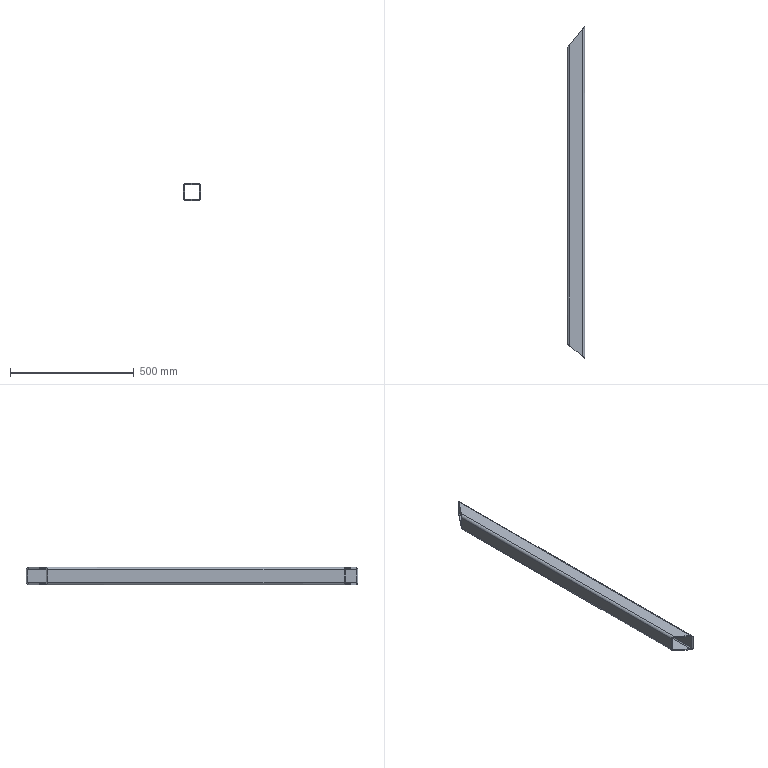Part | SolidWorks | features ICE 1, WeldMemberFeat 1, WeldmentFeature 1 | 1 solid | 18 faces | box 70 x 1340 x 70 mm | volume 1567074 mm3 | plane 10 | cylinder 8 | commonest cylinder face diameters 10 x4 20 x4
STEP:
#1=CARTESIAN_POINT('',(35.,0.,25.));
#2=VERTEX_POINT('',#1);
#3=CARTESIAN_POINT('',(35.,0.,-25.));
#4=VERTEX_POINT('',#3);
#5=CARTESIAN_POINT('',(35.,0.,-25.));
#6=DIRECTION('',(0.,0.,-1.));
#7=VECTOR('',#6,1000.);
#8=LINE('',#5,#7);
#9=EDGE_CURVE('',#2,#4,#8,.T.);
#10=ORIENTED_EDGE('',*,*,#9,.T.);
#11=CARTESIAN_POINT('',(35.,1340.,-25.));
#12=VERTEX_POINT('',#11);
#13=CARTESIAN_POINT('',(35.,1340.,-25.));
#14=DIRECTION('',(0.,-1.,0.));
#15=VECTOR('',#14,1000.);
#16=LINE('',#13,#15);
#17=EDGE_CURVE('',#12,#4,#16,.T.);
#18=ORIENTED_EDGE('',*,*,#17,.F.);
#19=CARTESIAN_POINT('',(35.,1340.,25.));
#20=VERTEX_POINT('',#19);
#21=CARTESIAN_POINT('',(35.,1340.,-25.));
#22=DIRECTION('',(0.,0.,-1.));
#23=VECTOR('',#22,1000.);
#24=LINE('',#21,#23);
#25=EDGE_CURVE('',#20,#12,#24,.T.);
#26=ORIENTED_EDGE('',*,*,#25,.F.);
#27=CARTESIAN_POINT('',(35.,1340.,25.));
#28=DIRECTION('',(0.,-1.,0.));
#29=VECTOR('',#28,1000.);
#30=LINE('',#27,#29);
#31=EDGE_CURVE('',#20,#2,#30,.T.);
#32=ORIENTED_EDGE('',*,*,#31,.T.);
#33=EDGE_LOOP('',(#10,#18,#26,#32));
#34=FACE_OUTER_BOUND('',#33,.T.);
#35=CARTESIAN_POINT('',(35.,1340.,-25.));
#36=DIRECTION('',(-1.,0.,0.));
#37=DIRECTION('',(0.,0.,1.));
#38=AXIS2_PLACEMENT_3D('',#35,#36,#37);
#39=PLANE('',#38);
#40=ADVANCED_FACE('',(#34),#39,.F.);
#41=CARTESIAN_POINT('',(-35.,1252.5,25.));
#42=VERTEX_POINT('',#41);
#43=CARTESIAN_POINT('',(-35.,56.,25.));
#44=VERTEX_POINT('',#43);
#45=CARTESIAN_POINT('',(-35.,1340.,25.));
#46=DIRECTION('',(0.,-1.,0.));
#47=VECTOR('',#46,1000.);
#48=LINE('',#45,#47);
#49=EDGE_CURVE('',#42,#44,#48,.T.);
#50=ORIENTED_EDGE('',*,*,#49,.F.);
#51=CARTESIAN_POINT('',(-35.,1252.5,-25.));
#52=VERTEX_POINT('',#51);
#53=CARTESIAN_POINT('',(-35.,1252.5,-35.));
#54=DIRECTION('',(0.,0.,1.));
#55=VECTOR('',#54,1000.);
#56=LINE('',#53,#55);
#57=EDGE_CURVE('',#52,#42,#56,.T.);
#58=ORIENTED_EDGE('',*,*,#57,.F.);
#59=CARTESIAN_POINT('',(-35.,56.,-25.));
#60=VERTEX_POINT('',#59);
#61=CARTESIAN_POINT('',(-35.,1340.,-25.));
#62=DIRECTION('',(0.,-1.,0.));
#63=VECTOR('',#62,1000.);
#64=LINE('',#61,#63);
#65=EDGE_CURVE('',#52,#60,#64,.T.);
#66=ORIENTED_EDGE('',*,*,#65,.T.);
#67=CARTESIAN_POINT('',(-35.,56.,-35.));
#68=DIRECTION('',(0.,0.,1.));
#69=VECTOR('',#68,1000.);
#70=LINE('',#67,#69);
#71=EDGE_CURVE('',#60,#44,#70,.T.);
#72=ORIENTED_EDGE('',*,*,#71,.T.);
#73=EDGE_LOOP('',(#50,#58,#66,#72));
#74=FACE_OUTER_BOUND('',#73,.T.);
#75=CARTESIAN_POINT('',(-35.,1340.,25.));
#76=DIRECTION('',(1.,0.,0.));
#77=DIRECTION('',(0.,0.,-1.));
#78=AXIS2_PLACEMENT_3D('',#75,#76,#77);
#79=PLANE('',#78);
#80=ADVANCED_FACE('',(#74),#79,.F.);
#81=ORIENTED_EDGE('',*,*,#65,.F.);
#82=CARTESIAN_POINT('',(-25.,1265.,-35.));
#83=VERTEX_POINT('',#82);
#84=CARTESIAN_POINT('',(-35.,1252.5,-25.));
#85=CARTESIAN_POINT('',(-35.,1252.5,-30.858));
#86=CARTESIAN_POINT('',(-30.858,1257.678,-35.));
#87=CARTESIAN_POINT('',(-25.,1265.,-35.));
#88=(BOUNDED_CURVE()B_SPLINE_CURVE(3,(#84,#85,#86,#87),.UNSPECIFIED.,.F.,.T.)B_SPLINE_CURVE_WITH_KNOTS((4,4),(0.,1.571),.UNSPECIFIED.)CURVE()GEOMETRIC_REPRESENTATION_ITEM()RATIONAL_B_SPLINE_CURVE((1.,0.8047,0.8047,1.))REPRESENTATION_ITEM(''));
#89=EDGE_CURVE('',#52,#83,#88,.T.);
#90=ORIENTED_EDGE('',*,*,#89,.T.);
#91=CARTESIAN_POINT('',(-25.,48.,-35.));
#92=VERTEX_POINT('',#91);
#93=CARTESIAN_POINT('',(-25.,1340.,-35.));
#94=DIRECTION('',(0.,-1.,0.));
#95=VECTOR('',#94,1000.);
#96=LINE('',#93,#95);
#97=EDGE_CURVE('',#83,#92,#96,.T.);
#98=ORIENTED_EDGE('',*,*,#97,.T.);
#99=CARTESIAN_POINT('',(-25.,48.,-35.));
#100=CARTESIAN_POINT('',(-30.858,52.686,-35.));
#101=CARTESIAN_POINT('',(-35.,56.,-30.858));
#102=CARTESIAN_POINT('',(-35.,56.,-25.));
#103=(BOUNDED_CURVE()B_SPLINE_CURVE(3,(#99,#100,#101,#102),.UNSPECIFIED.,.F.,.T.)B_SPLINE_CURVE_WITH_KNOTS((4,4),(1.571,3.142),.UNSPECIFIED.)CURVE()GEOMETRIC_REPRESENTATION_ITEM()RATIONAL_B_SPLINE_CURVE((1.,0.8047,0.8047,1.))REPRESENTATION_ITEM(''));
#104=EDGE_CURVE('',#92,#60,#103,.T.);
#105=ORIENTED_EDGE('',*,*,#104,.T.);
#106=EDGE_LOOP('',(#81,#90,#98,#105));
#107=FACE_OUTER_BOUND('',#106,.T.);
#108=CARTESIAN_POINT('',(-25.,1340.,-25.));
#109=DIRECTION('',(0.,-1.,0.));
#110=DIRECTION('',(0.,0.,-1.));
#111=AXIS2_PLACEMENT_3D('',#108,#109,#110);
#112=CYLINDRICAL_SURFACE('',#111,10.);
#113=ADVANCED_FACE('',(#107),#112,.T.);
#114=ORIENTED_EDGE('',*,*,#97,.F.);
#115=CARTESIAN_POINT('',(25.,1327.5,-35.));
#116=VERTEX_POINT('',#115);
#117=CARTESIAN_POINT('',(35.,1340.,-35.));
#118=DIRECTION('',(0.6247,0.7809,0.));
#119=VECTOR('',#118,1000.);
#120=LINE('',#117,#119);
#121=EDGE_CURVE('',#83,#116,#120,.T.);
#122=ORIENTED_EDGE('',*,*,#121,.T.);
#123=CARTESIAN_POINT('',(25.,8.,-35.));
#124=VERTEX_POINT('',#123);
#125=CARTESIAN_POINT('',(25.,1340.,-35.));
#126=DIRECTION('',(0.,-1.,0.));
#127=VECTOR('',#126,1000.);
#128=LINE('',#125,#127);
#129=EDGE_CURVE('',#116,#124,#128,.T.);
#130=ORIENTED_EDGE('',*,*,#129,.T.);
#131=CARTESIAN_POINT('',(-35.,56.,-35.));
#132=DIRECTION('',(-0.7809,0.6247,0.));
#133=VECTOR('',#132,1000.);
#134=LINE('',#131,#133);
#135=EDGE_CURVE('',#124,#92,#134,.T.);
#136=ORIENTED_EDGE('',*,*,#135,.T.);
#137=EDGE_LOOP('',(#114,#122,#130,#136));
#138=FACE_OUTER_BOUND('',#137,.T.);
#139=CARTESIAN_POINT('',(25.,1340.,-35.));
#140=DIRECTION('',(0.,0.,1.));
#141=DIRECTION('',(1.,0.,0.));
#142=AXIS2_PLACEMENT_3D('',#139,#140,#141);
#143=PLANE('',#142);
#144=ADVANCED_FACE('',(#138),#143,.F.);
#145=ORIENTED_EDGE('',*,*,#129,.F.);
#146=CARTESIAN_POINT('',(25.,1327.5,-35.));
#147=CARTESIAN_POINT('',(30.858,1334.822,-35.));
#148=CARTESIAN_POINT('',(35.,1340.,-30.858));
#149=CARTESIAN_POINT('',(35.,1340.,-25.));
#150=(BOUNDED_CURVE()B_SPLINE_CURVE(3,(#146,#147,#148,#149),.UNSPECIFIED.,.F.,.F.)B_SPLINE_CURVE_WITH_KNOTS((4,4),(1.571,3.142),.UNSPECIFIED.)CURVE()GEOMETRIC_REPRESENTATION_ITEM()RATIONAL_B_SPLINE_CURVE((1.,0.8047,0.8047,1.))REPRESENTATION_ITEM(''));
#151=EDGE_CURVE('',#116,#12,#150,.T.);
#152=ORIENTED_EDGE('',*,*,#151,.T.);
#153=ORIENTED_EDGE('',*,*,#17,.T.);
#154=CARTESIAN_POINT('',(35.,0.,-25.));
#155=CARTESIAN_POINT('',(35.,0.,-30.858));
#156=CARTESIAN_POINT('',(30.858,3.314,-35.));
#157=CARTESIAN_POINT('',(25.,8.,-35.));
#158=(BOUNDED_CURVE()B_SPLINE_CURVE(3,(#154,#155,#156,#157),.UNSPECIFIED.,.F.,.F.)B_SPLINE_CURVE_WITH_KNOTS((4,4),(0.,1.571),.UNSPECIFIED.)CURVE()GEOMETRIC_REPRESENTATION_ITEM()RATIONAL_B_SPLINE_CURVE((1.,0.8047,0.8047,1.))REPRESENTATION_ITEM(''));
#159=EDGE_CURVE('',#4,#124,#158,.T.);
#160=ORIENTED_EDGE('',*,*,#159,.T.);
#161=EDGE_LOOP('',(#145,#152,#153,#160));
#162=FACE_OUTER_BOUND('',#161,.T.);
#163=CARTESIAN_POINT('',(25.,1340.,-25.));
#164=DIRECTION('',(0.,-1.,0.));
#165=DIRECTION('',(0.,0.,-1.));
#166=AXIS2_PLACEMENT_3D('',#163,#164,#165);
#167=CYLINDRICAL_SURFACE('',#166,10.);
#168=ADVANCED_FACE('',(#162),#167,.T.);
#169=ORIENTED_EDGE('',*,*,#31,.F.);
#170=CARTESIAN_POINT('',(25.,1327.5,35.));
#171=VERTEX_POINT('',#170);
#172=CARTESIAN_POINT('',(35.,1340.,25.));
#173=CARTESIAN_POINT('',(35.,1340.,30.858));
#174=CARTESIAN_POINT('',(30.858,1334.822,35.));
#175=CARTESIAN_POINT('',(25.,1327.5,35.));
#176=(BOUNDED_CURVE()B_SPLINE_CURVE(3,(#172,#173,#174,#175),.UNSPECIFIED.,.F.,.T.)B_SPLINE_CURVE_WITH_KNOTS((4,4),(3.142,4.712),.UNSPECIFIED.)CURVE()GEOMETRIC_REPRESENTATION_ITEM()RATIONAL_B_SPLINE_CURVE((1.,0.8047,0.8047,1.))REPRESENTATION_ITEM(''));
#177=EDGE_CURVE('',#20,#171,#176,.T.);
#178=ORIENTED_EDGE('',*,*,#177,.T.);
#179=CARTESIAN_POINT('',(25.,8.,35.));
#180=VERTEX_POINT('',#179);
#181=CARTESIAN_POINT('',(25.,1340.,35.));
#182=DIRECTION('',(0.,-1.,0.));
#183=VECTOR('',#182,1000.);
#184=LINE('',#181,#183);
#185=EDGE_CURVE('',#171,#180,#184,.T.);
#186=ORIENTED_EDGE('',*,*,#185,.T.);
#187=CARTESIAN_POINT('',(25.,8.,35.));
#188=CARTESIAN_POINT('',(30.858,3.314,35.));
#189=CARTESIAN_POINT('',(35.,0.,30.858));
#190=CARTESIAN_POINT('',(35.,0.,25.));
#191=(BOUNDED_CURVE()B_SPLINE_CURVE(3,(#187,#188,#189,#190),.UNSPECIFIED.,.F.,.F.)B_SPLINE_CURVE_WITH_KNOTS((4,4),(4.712,6.283),.UNSPECIFIED.)CURVE()GEOMETRIC_REPRESENTATION_ITEM()RATIONAL_B_SPLINE_CURVE((1.,0.8047,0.8047,1.))REPRESENTATION_ITEM(''));
#192=EDGE_CURVE('',#180,#2,#191,.T.);
#193=ORIENTED_EDGE('',*,*,#192,.T.);
#194=EDGE_LOOP('',(#169,#178,#186,#193));
#195=FACE_OUTER_BOUND('',#194,.T.);
#196=CARTESIAN_POINT('',(25.,1340.,25.));
#197=DIRECTION('',(0.,-1.,0.));
#198=DIRECTION('',(0.,0.,-1.));
#199=AXIS2_PLACEMENT_3D('',#196,#197,#198);
#200=CYLINDRICAL_SURFACE('',#199,10.);
#201=ADVANCED_FACE('',(#195),#200,.T.);
#202=ORIENTED_EDGE('',*,*,#185,.F.);
#203=CARTESIAN_POINT('',(-25.,1265.,35.));
#204=VERTEX_POINT('',#203);
#205=CARTESIAN_POINT('',(11.585,1310.732,35.));
#206=DIRECTION('',(-0.6247,-0.7809,0.));
#207=VECTOR('',#206,1000.);
#208=LINE('',#205,#207);
#209=EDGE_CURVE('',#171,#204,#208,.T.);
#210=ORIENTED_EDGE('',*,*,#209,.T.);
#211=CARTESIAN_POINT('',(-25.,48.,35.));
#212=VERTEX_POINT('',#211);
#213=CARTESIAN_POINT('',(-25.,1340.,35.));
#214=DIRECTION('',(0.,-1.,0.));
#215=VECTOR('',#214,1000.);
#216=LINE('',#213,#215);
#217=EDGE_CURVE('',#204,#212,#216,.T.);
#218=ORIENTED_EDGE('',*,*,#217,.T.);
#219=CARTESIAN_POINT('',(-655.244,552.195,35.));
#220=DIRECTION('',(0.7809,-0.6247,0.));
#221=VECTOR('',#220,1000.);
#222=LINE('',#219,#221);
#223=EDGE_CURVE('',#212,#180,#222,.T.);
#224=ORIENTED_EDGE('',*,*,#223,.T.);
#225=EDGE_LOOP('',(#202,#210,#218,#224));
#226=FACE_OUTER_BOUND('',#225,.T.);
#227=CARTESIAN_POINT('',(-25.,1340.,35.));
#228=DIRECTION('',(0.,0.,-1.));
#229=DIRECTION('',(-1.,0.,0.));
#230=AXIS2_PLACEMENT_3D('',#227,#228,#229);
#231=PLANE('',#230);
#232=ADVANCED_FACE('',(#226),#231,.F.);
#233=ORIENTED_EDGE('',*,*,#217,.F.);
#234=CARTESIAN_POINT('',(-25.,1265.,35.));
#235=CARTESIAN_POINT('',(-30.858,1257.678,35.));
#236=CARTESIAN_POINT('',(-35.,1252.5,30.858));
#237=CARTESIAN_POINT('',(-35.,1252.5,25.));
#238=(BOUNDED_CURVE()B_SPLINE_CURVE(3,(#234,#235,#236,#237),.UNSPECIFIED.,.F.,.F.)B_SPLINE_CURVE_WITH_KNOTS((4,4),(4.712,6.283),.UNSPECIFIED.)CURVE()GEOMETRIC_REPRESENTATION_ITEM()RATIONAL_B_SPLINE_CURVE((1.,0.8047,0.8047,1.))REPRESENTATION_ITEM(''));
#239=EDGE_CURVE('',#204,#42,#238,.T.);
#240=ORIENTED_EDGE('',*,*,#239,.T.);
#241=ORIENTED_EDGE('',*,*,#49,.T.);
#242=CARTESIAN_POINT('',(-35.,56.,25.));
#243=CARTESIAN_POINT('',(-35.,56.,30.858));
#244=CARTESIAN_POINT('',(-30.858,52.686,35.));
#245=CARTESIAN_POINT('',(-25.,48.,35.));
#246=(BOUNDED_CURVE()B_SPLINE_CURVE(3,(#242,#243,#244,#245),.UNSPECIFIED.,.F.,.F.)B_SPLINE_CURVE_WITH_KNOTS((4,4),(3.142,4.712),.UNSPECIFIED.)CURVE()GEOMETRIC_REPRESENTATION_ITEM()RATIONAL_B_SPLINE_CURVE((1.,0.8047,0.8047,1.))REPRESENTATION_ITEM(''));
#247=EDGE_CURVE('',#44,#212,#246,.T.);
#248=ORIENTED_EDGE('',*,*,#247,.T.);
#249=EDGE_LOOP('',(#233,#240,#241,#248));
#250=FACE_OUTER_BOUND('',#249,.T.);
#251=CARTESIAN_POINT('',(-25.,1340.,25.));
#252=DIRECTION('',(0.,-1.,0.));
#253=DIRECTION('',(0.,0.,-1.));
#254=AXIS2_PLACEMENT_3D('',#251,#252,#253);
#255=CYLINDRICAL_SURFACE('',#254,10.);
#256=ADVANCED_FACE('',(#250),#255,.T.);
#257=CARTESIAN_POINT('',(25.,8.,30.));
#258=VERTEX_POINT('',#257);
#259=CARTESIAN_POINT('',(30.,4.,25.));
#260=VERTEX_POINT('',#259);
#261=CARTESIAN_POINT('',(25.,8.,30.));
#262=CARTESIAN_POINT('',(27.929,5.657,30.));
#263=CARTESIAN_POINT('',(30.,4.,27.929));
#264=CARTESIAN_POINT('',(30.,4.,25.));
#265=(BOUNDED_CURVE()B_SPLINE_CURVE(3,(#261,#262,#263,#264),.UNSPECIFIED.,.F.,.F.)B_SPLINE_CURVE_WITH_KNOTS((4,4),(4.712,6.283),.UNSPECIFIED.)CURVE()GEOMETRIC_REPRESENTATION_ITEM()RATIONAL_B_SPLINE_CURVE((1.,0.8047,0.8047,1.))REPRESENTATION_ITEM(''));
#266=EDGE_CURVE('',#258,#260,#265,.T.);
#267=ORIENTED_EDGE('',*,*,#266,.T.);
#268=CARTESIAN_POINT('',(30.,4.,-25.));
#269=VERTEX_POINT('',#268);
#270=CARTESIAN_POINT('',(30.,4.,-25.));
#271=DIRECTION('',(0.,0.,-1.));
#272=VECTOR('',#271,1000.);
#273=LINE('',#270,#272);
#274=EDGE_CURVE('',#260,#269,#273,.T.);
#275=ORIENTED_EDGE('',*,*,#274,.T.);
#276=CARTESIAN_POINT('',(25.,8.,-30.));
#277=VERTEX_POINT('',#276);
#278=CARTESIAN_POINT('',(30.,4.,-25.));
#279=CARTESIAN_POINT('',(30.,4.,-27.929));
#280=CARTESIAN_POINT('',(27.929,5.657,-30.));
#281=CARTESIAN_POINT('',(25.,8.,-30.));
#282=(BOUNDED_CURVE()B_SPLINE_CURVE(3,(#278,#279,#280,#281),.UNSPECIFIED.,.F.,.F.)B_SPLINE_CURVE_WITH_KNOTS((4,4),(0.,1.571),.UNSPECIFIED.)CURVE()GEOMETRIC_REPRESENTATION_ITEM()RATIONAL_B_SPLINE_CURVE((1.,0.8047,0.8047,1.))REPRESENTATION_ITEM(''));
#283=EDGE_CURVE('',#269,#277,#282,.T.);
#284=ORIENTED_EDGE('',*,*,#283,.T.);
#285=CARTESIAN_POINT('',(-25.,48.,-30.));
#286=VERTEX_POINT('',#285);
#287=CARTESIAN_POINT('',(-624.756,527.805,-30.));
#288=DIRECTION('',(-0.7809,0.6247,0.));
#289=VECTOR('',#288,1000.);
#290=LINE('',#287,#289);
#291=EDGE_CURVE('',#277,#286,#290,.T.);
#292=ORIENTED_EDGE('',*,*,#291,.T.);
#293=CARTESIAN_POINT('',(-30.,52.,-25.));
#294=VERTEX_POINT('',#293);
#295=CARTESIAN_POINT('',(-25.,48.,-30.));
#296=CARTESIAN_POINT('',(-27.929,50.343,-30.));
#297=CARTESIAN_POINT('',(-30.,52.,-27.929));
#298=CARTESIAN_POINT('',(-30.,52.,-25.));
#299=(BOUNDED_CURVE()B_SPLINE_CURVE(3,(#295,#296,#297,#298),.UNSPECIFIED.,.F.,.F.)B_SPLINE_CURVE_WITH_KNOTS((4,4),(1.571,3.142),.UNSPECIFIED.)CURVE()GEOMETRIC_REPRESENTATION_ITEM()RATIONAL_B_SPLINE_CURVE((1.,0.8047,0.8047,1.))REPRESENTATION_ITEM(''));
#300=EDGE_CURVE('',#286,#294,#299,.T.);
#301=ORIENTED_EDGE('',*,*,#300,.T.);
#302=CARTESIAN_POINT('',(-30.,52.,25.));
#303=VERTEX_POINT('',#302);
#304=CARTESIAN_POINT('',(-30.,52.,25.));
#305=DIRECTION('',(0.,0.,1.));
#306=VECTOR('',#305,1000.);
#307=LINE('',#304,#306);
#308=EDGE_CURVE('',#294,#303,#307,.T.);
#309=ORIENTED_EDGE('',*,*,#308,.T.);
#310=CARTESIAN_POINT('',(-25.,48.,30.));
#311=VERTEX_POINT('',#310);
#312=CARTESIAN_POINT('',(-30.,52.,25.));
#313=CARTESIAN_POINT('',(-30.,52.,27.929));
#314=CARTESIAN_POINT('',(-27.929,50.343,30.));
#315=CARTESIAN_POINT('',(-25.,48.,30.));
#316=(BOUNDED_CURVE()B_SPLINE_CURVE(3,(#312,#313,#314,#315),.UNSPECIFIED.,.F.,.T.)B_SPLINE_CURVE_WITH_KNOTS((4,4),(3.142,4.712),.UNSPECIFIED.)CURVE()GEOMETRIC_REPRESENTATION_ITEM()RATIONAL_B_SPLINE_CURVE((1.,0.8047,0.8047,1.))REPRESENTATION_ITEM(''));
#317=EDGE_CURVE('',#303,#311,#316,.T.);
#318=ORIENTED_EDGE('',*,*,#317,.T.);
#319=CARTESIAN_POINT('',(-655.244,552.195,30.));
#320=DIRECTION('',(0.7809,-0.6247,0.));
#321=VECTOR('',#320,1000.);
#322=LINE('',#319,#321);
#323=EDGE_CURVE('',#311,#258,#322,.T.);
#324=ORIENTED_EDGE('',*,*,#323,.T.);
#325=EDGE_LOOP('',(#267,#275,#284,#292,#301,#309,#318,#324));
#326=FACE_BOUND('',#325,.T.);
#327=ORIENTED_EDGE('',*,*,#71,.F.);
#328=ORIENTED_EDGE('',*,*,#104,.F.);
#329=ORIENTED_EDGE('',*,*,#135,.F.);
#330=ORIENTED_EDGE('',*,*,#159,.F.);
#331=ORIENTED_EDGE('',*,*,#9,.F.);
#332=ORIENTED_EDGE('',*,*,#192,.F.);
#333=ORIENTED_EDGE('',*,*,#223,.F.);
#334=ORIENTED_EDGE('',*,*,#247,.F.);
#335=EDGE_LOOP('',(#327,#328,#329,#330,#331,#332,#333,#334));
#336=FACE_OUTER_BOUND('',#335,.T.);
#337=CARTESIAN_POINT('',(-35.,56.,-35.));
#338=DIRECTION('',(0.6247,0.7809,0.));
#339=DIRECTION('',(-0.7809,0.6247,0.));
#340=AXIS2_PLACEMENT_3D('',#337,#338,#339);
#341=PLANE('',#340);
#342=ADVANCED_FACE('',(#326,#336),#341,.F.);
#343=CARTESIAN_POINT('',(30.,1333.75,25.));
#344=VERTEX_POINT('',#343);
#345=CARTESIAN_POINT('',(25.,1327.5,30.));
#346=VERTEX_POINT('',#345);
#347=CARTESIAN_POINT('',(30.,1333.75,25.));
#348=CARTESIAN_POINT('',(30.,1333.75,27.929));
#349=CARTESIAN_POINT('',(27.929,1331.161,30.));
#350=CARTESIAN_POINT('',(25.,1327.5,30.));
#351=(BOUNDED_CURVE()B_SPLINE_CURVE(3,(#347,#348,#349,#350),.UNSPECIFIED.,.F.,.T.)B_SPLINE_CURVE_WITH_KNOTS((4,4),(3.142,4.712),.UNSPECIFIED.)CURVE()GEOMETRIC_REPRESENTATION_ITEM()RATIONAL_B_SPLINE_CURVE((1.,0.8047,0.8047,1.))REPRESENTATION_ITEM(''));
#352=EDGE_CURVE('',#344,#346,#351,.T.);
#353=ORIENTED_EDGE('',*,*,#352,.T.);
#354=CARTESIAN_POINT('',(-25.,1265.,30.));
#355=VERTEX_POINT('',#354);
#356=CARTESIAN_POINT('',(11.585,1310.732,30.));
#357=DIRECTION('',(-0.6247,-0.7809,0.));
#358=VECTOR('',#357,1000.);
#359=LINE('',#356,#358);
#360=EDGE_CURVE('',#346,#355,#359,.T.);
#361=ORIENTED_EDGE('',*,*,#360,.T.);
#362=CARTESIAN_POINT('',(-30.,1258.75,25.));
#363=VERTEX_POINT('',#362);
#364=CARTESIAN_POINT('',(-25.,1265.,30.));
#365=CARTESIAN_POINT('',(-27.929,1261.339,30.));
#366=CARTESIAN_POINT('',(-30.,1258.75,27.929));
#367=CARTESIAN_POINT('',(-30.,1258.75,25.));
#368=(BOUNDED_CURVE()B_SPLINE_CURVE(3,(#364,#365,#366,#367),.UNSPECIFIED.,.F.,.F.)B_SPLINE_CURVE_WITH_KNOTS((4,4),(4.712,6.283),.UNSPECIFIED.)CURVE()GEOMETRIC_REPRESENTATION_ITEM()RATIONAL_B_SPLINE_CURVE((1.,0.8047,0.8047,1.))REPRESENTATION_ITEM(''));
#369=EDGE_CURVE('',#355,#363,#368,.T.);
#370=ORIENTED_EDGE('',*,*,#369,.T.);
#371=CARTESIAN_POINT('',(-30.,1258.75,-25.));
#372=VERTEX_POINT('',#371);
#373=CARTESIAN_POINT('',(-30.,1258.75,25.));
#374=DIRECTION('',(0.,0.,-1.));
#375=VECTOR('',#374,1000.);
#376=LINE('',#373,#375);
#377=EDGE_CURVE('',#363,#372,#376,.T.);
#378=ORIENTED_EDGE('',*,*,#377,.T.);
#379=CARTESIAN_POINT('',(-25.,1265.,-30.));
#380=VERTEX_POINT('',#379);
#381=CARTESIAN_POINT('',(-30.,1258.75,-25.));
#382=CARTESIAN_POINT('',(-30.,1258.75,-27.929));
#383=CARTESIAN_POINT('',(-27.929,1261.339,-30.));
#384=CARTESIAN_POINT('',(-25.,1265.,-30.));
#385=(BOUNDED_CURVE()B_SPLINE_CURVE(3,(#381,#382,#383,#384),.UNSPECIFIED.,.F.,.F.)B_SPLINE_CURVE_WITH_KNOTS((4,4),(0.,1.571),.UNSPECIFIED.)CURVE()GEOMETRIC_REPRESENTATION_ITEM()RATIONAL_B_SPLINE_CURVE((1.,0.8047,0.8047,1.))REPRESENTATION_ITEM(''));
#386=EDGE_CURVE('',#372,#380,#385,.T.);
#387=ORIENTED_EDGE('',*,*,#386,.T.);
#388=CARTESIAN_POINT('',(25.,1327.5,-30.));
#389=VERTEX_POINT('',#388);
#390=CARTESIAN_POINT('',(31.098,1335.122,-30.));
#391=DIRECTION('',(0.6247,0.7809,0.));
#392=VECTOR('',#391,1000.);
#393=LINE('',#390,#392);
#394=EDGE_CURVE('',#380,#389,#393,.T.);
#395=ORIENTED_EDGE('',*,*,#394,.T.);
#396=CARTESIAN_POINT('',(30.,1333.75,-25.));
#397=VERTEX_POINT('',#396);
#398=CARTESIAN_POINT('',(25.,1327.5,-30.));
#399=CARTESIAN_POINT('',(27.929,1331.161,-30.));
#400=CARTESIAN_POINT('',(30.,1333.75,-27.929));
#401=CARTESIAN_POINT('',(30.,1333.75,-25.));
#402=(BOUNDED_CURVE()B_SPLINE_CURVE(3,(#398,#399,#400,#401),.UNSPECIFIED.,.F.,.F.)B_SPLINE_CURVE_WITH_KNOTS((4,4),(1.571,3.142),.UNSPECIFIED.)CURVE()GEOMETRIC_REPRESENTATION_ITEM()RATIONAL_B_SPLINE_CURVE((1.,0.8047,0.8047,1.))REPRESENTATION_ITEM(''));
#403=EDGE_CURVE('',#389,#397,#402,.T.);
#404=ORIENTED_EDGE('',*,*,#403,.T.);
#405=CARTESIAN_POINT('',(30.,1333.75,-25.));
#406=DIRECTION('',(0.,0.,1.));
#407=VECTOR('',#406,1000.);
#408=LINE('',#405,#407);
#409=EDGE_CURVE('',#397,#344,#408,.T.);
#410=ORIENTED_EDGE('',*,*,#409,.T.);
#411=EDGE_LOOP('',(#353,#361,#370,#378,#387,#395,#404,#410));
#412=FACE_BOUND('',#411,.T.);
#413=ORIENTED_EDGE('',*,*,#209,.F.);
#414=ORIENTED_EDGE('',*,*,#177,.F.);
#415=ORIENTED_EDGE('',*,*,#25,.T.);
#416=ORIENTED_EDGE('',*,*,#151,.F.);
#417=ORIENTED_EDGE('',*,*,#121,.F.);
#418=ORIENTED_EDGE('',*,*,#89,.F.);
#419=ORIENTED_EDGE('',*,*,#57,.T.);
#420=ORIENTED_EDGE('',*,*,#239,.F.);
#421=EDGE_LOOP('',(#413,#414,#415,#416,#417,#418,#419,#420));
#422=FACE_OUTER_BOUND('',#421,.T.);
#423=CARTESIAN_POINT('',(35.,1340.,-35.));
#424=DIRECTION('',(0.7809,-0.6247,0.));
#425=DIRECTION('',(0.6247,0.7809,0.));
#426=AXIS2_PLACEMENT_3D('',#423,#424,#425);
#427=PLANE('',#426);
#428=ADVANCED_FACE('',(#412,#422),#427,.F.);
#429=ORIENTED_EDGE('',*,*,#352,.F.);
#430=CARTESIAN_POINT('',(30.,1340.,25.));
#431=DIRECTION('',(0.,-1.,0.));
#432=VECTOR('',#431,1000.);
#433=LINE('',#430,#432);
#434=EDGE_CURVE('',#344,#260,#433,.T.);
#435=ORIENTED_EDGE('',*,*,#434,.T.);
#436=ORIENTED_EDGE('',*,*,#266,.F.);
#437=CARTESIAN_POINT('',(25.,1340.,30.));
#438=DIRECTION('',(0.,-1.,0.));
#439=VECTOR('',#438,1000.);
#440=LINE('',#437,#439);
#441=EDGE_CURVE('',#346,#258,#440,.T.);
#442=ORIENTED_EDGE('',*,*,#441,.F.);
#443=EDGE_LOOP('',(#429,#435,#436,#442));
#444=FACE_OUTER_BOUND('',#443,.T.);
#445=CARTESIAN_POINT('',(25.,1340.,25.));
#446=DIRECTION('',(0.,-1.,0.));
#447=DIRECTION('',(0.,0.,-1.));
#448=AXIS2_PLACEMENT_3D('',#445,#446,#447);
#449=CYLINDRICAL_SURFACE('',#448,5.);
#450=ADVANCED_FACE('',(#444),#449,.F.);
#451=ORIENTED_EDGE('',*,*,#360,.F.);
#452=ORIENTED_EDGE('',*,*,#441,.T.);
#453=ORIENTED_EDGE('',*,*,#323,.F.);
#454=CARTESIAN_POINT('',(-25.,1340.,30.));
#455=DIRECTION('',(0.,-1.,0.));
#456=VECTOR('',#455,1000.);
#457=LINE('',#454,#456);
#458=EDGE_CURVE('',#355,#311,#457,.T.);
#459=ORIENTED_EDGE('',*,*,#458,.F.);
#460=EDGE_LOOP('',(#451,#452,#453,#459));
#461=FACE_OUTER_BOUND('',#460,.T.);
#462=CARTESIAN_POINT('',(-25.,1340.,30.));
#463=DIRECTION('',(0.,0.,-1.));
#464=DIRECTION('',(-1.,0.,0.));
#465=AXIS2_PLACEMENT_3D('',#462,#463,#464);
#466=PLANE('',#465);
#467=ADVANCED_FACE('',(#461),#466,.T.);
#468=ORIENTED_EDGE('',*,*,#369,.F.);
#469=ORIENTED_EDGE('',*,*,#458,.T.);
#470=ORIENTED_EDGE('',*,*,#317,.F.);
#471=CARTESIAN_POINT('',(-30.,1340.,25.));
#472=DIRECTION('',(0.,-1.,0.));
#473=VECTOR('',#472,1000.);
#474=LINE('',#471,#473);
#475=EDGE_CURVE('',#363,#303,#474,.T.);
#476=ORIENTED_EDGE('',*,*,#475,.F.);
#477=EDGE_LOOP('',(#468,#469,#470,#476));
#478=FACE_OUTER_BOUND('',#477,.T.);
#479=CARTESIAN_POINT('',(-25.,1340.,25.));
#480=DIRECTION('',(0.,-1.,0.));
#481=DIRECTION('',(0.,0.,-1.));
#482=AXIS2_PLACEMENT_3D('',#479,#480,#481);
#483=CYLINDRICAL_SURFACE('',#482,5.);
#484=ADVANCED_FACE('',(#478),#483,.F.);
#485=ORIENTED_EDGE('',*,*,#377,.F.);
#486=ORIENTED_EDGE('',*,*,#475,.T.);
#487=ORIENTED_EDGE('',*,*,#308,.F.);
#488=CARTESIAN_POINT('',(-30.,1340.,-25.));
#489=DIRECTION('',(0.,-1.,0.));
#490=VECTOR('',#489,1000.);
#491=LINE('',#488,#490);
#492=EDGE_CURVE('',#372,#294,#491,.T.);
#493=ORIENTED_EDGE('',*,*,#492,.F.);
#494=EDGE_LOOP('',(#485,#486,#487,#493));
#495=FACE_OUTER_BOUND('',#494,.T.);
#496=CARTESIAN_POINT('',(-30.,1340.,25.));
#497=DIRECTION('',(1.,0.,0.));
#498=DIRECTION('',(0.,0.,-1.));
#499=AXIS2_PLACEMENT_3D('',#496,#497,#498);
#500=PLANE('',#499);
#501=ADVANCED_FACE('',(#495),#500,.T.);
#502=ORIENTED_EDGE('',*,*,#386,.F.);
#503=ORIENTED_EDGE('',*,*,#492,.T.);
#504=ORIENTED_EDGE('',*,*,#300,.F.);
#505=CARTESIAN_POINT('',(-25.,1340.,-30.));
#506=DIRECTION('',(0.,-1.,0.));
#507=VECTOR('',#506,1000.);
#508=LINE('',#505,#507);
#509=EDGE_CURVE('',#380,#286,#508,.T.);
#510=ORIENTED_EDGE('',*,*,#509,.F.);
#511=EDGE_LOOP('',(#502,#503,#504,#510));
#512=FACE_OUTER_BOUND('',#511,.T.);
#513=CARTESIAN_POINT('',(-25.,1340.,-25.));
#514=DIRECTION('',(0.,-1.,0.));
#515=DIRECTION('',(0.,0.,-1.));
#516=AXIS2_PLACEMENT_3D('',#513,#514,#515);
#517=CYLINDRICAL_SURFACE('',#516,5.);
#518=ADVANCED_FACE('',(#512),#517,.F.);
#519=ORIENTED_EDGE('',*,*,#394,.F.);
#520=ORIENTED_EDGE('',*,*,#509,.T.);
#521=ORIENTED_EDGE('',*,*,#291,.F.);
#522=CARTESIAN_POINT('',(25.,1340.,-30.));
#523=DIRECTION('',(0.,-1.,0.));
#524=VECTOR('',#523,1000.);
#525=LINE('',#522,#524);
#526=EDGE_CURVE('',#389,#277,#525,.T.);
#527=ORIENTED_EDGE('',*,*,#526,.F.);
#528=EDGE_LOOP('',(#519,#520,#521,#527));
#529=FACE_OUTER_BOUND('',#528,.T.);
#530=CARTESIAN_POINT('',(25.,1340.,-30.));
#531=DIRECTION('',(0.,0.,1.));
#532=DIRECTION('',(1.,0.,0.));
#533=AXIS2_PLACEMENT_3D('',#530,#531,#532);
#534=PLANE('',#533);
#535=ADVANCED_FACE('',(#529),#534,.T.);
#536=ORIENTED_EDGE('',*,*,#403,.F.);
#537=ORIENTED_EDGE('',*,*,#526,.T.);
#538=ORIENTED_EDGE('',*,*,#283,.F.);
#539=CARTESIAN_POINT('',(30.,1340.,-25.));
#540=DIRECTION('',(0.,-1.,0.));
#541=VECTOR('',#540,1000.);
#542=LINE('',#539,#541);
#543=EDGE_CURVE('',#397,#269,#542,.T.);
#544=ORIENTED_EDGE('',*,*,#543,.F.);
#545=EDGE_LOOP('',(#536,#537,#538,#544));
#546=FACE_OUTER_BOUND('',#545,.T.);
#547=CARTESIAN_POINT('',(25.,1340.,-25.));
#548=DIRECTION('',(0.,-1.,0.));
#549=DIRECTION('',(0.,0.,-1.));
#550=AXIS2_PLACEMENT_3D('',#547,#548,#549);
#551=CYLINDRICAL_SURFACE('',#550,5.);
#552=ADVANCED_FACE('',(#546),#551,.F.);
#553=ORIENTED_EDGE('',*,*,#409,.F.);
#554=ORIENTED_EDGE('',*,*,#543,.T.);
#555=ORIENTED_EDGE('',*,*,#274,.F.);
#556=ORIENTED_EDGE('',*,*,#434,.F.);
#557=EDGE_LOOP('',(#553,#554,#555,#556));
#558=FACE_OUTER_BOUND('',#557,.T.);
#559=CARTESIAN_POINT('',(30.,1340.,-25.));
#560=DIRECTION('',(-1.,0.,0.));
#561=DIRECTION('',(0.,0.,1.));
#562=AXIS2_PLACEMENT_3D('',#559,#560,#561);
#563=PLANE('',#562);
#564=ADVANCED_FACE('',(#558),#563,.T.);
#565=CLOSED_SHELL('',(#40,#80,#113,#144,#168,#201,#232,#256,#342,#428,#450,#467,#484,#501,#518,#535,#552,#564));
#566=MANIFOLD_SOLID_BREP('',#565);
#567=CARTESIAN_POINT('',(0.,0.,0.));
#568=DIRECTION('',(0.,0.,1.));
#569=DIRECTION('',(1.,0.,0.));
#570=AXIS2_PLACEMENT_3D('',#567,#568,#569);
#571=(LENGTH_UNIT()NAMED_UNIT(*)SI_UNIT(.MILLI.,.METRE.));
#572=UNCERTAINTY_MEASURE_WITH_UNIT(LENGTH_MEASURE(0.00001),#571,'','');
#573=(NAMED_UNIT(*)PLANE_ANGLE_UNIT()SI_UNIT($,.RADIAN.));
#574=(NAMED_UNIT(*)SI_UNIT($,.STERADIAN.)SOLID_ANGLE_UNIT());
#575=(GEOMETRIC_REPRESENTATION_CONTEXT(3)GLOBAL_UNCERTAINTY_ASSIGNED_CONTEXT((#572))GLOBAL_UNIT_ASSIGNED_CONTEXT((#571,#573,#574))REPRESENTATION_CONTEXT('',''));
#576=ADVANCED_BREP_SHAPE_REPRESENTATION('',(#566,#570),#575);